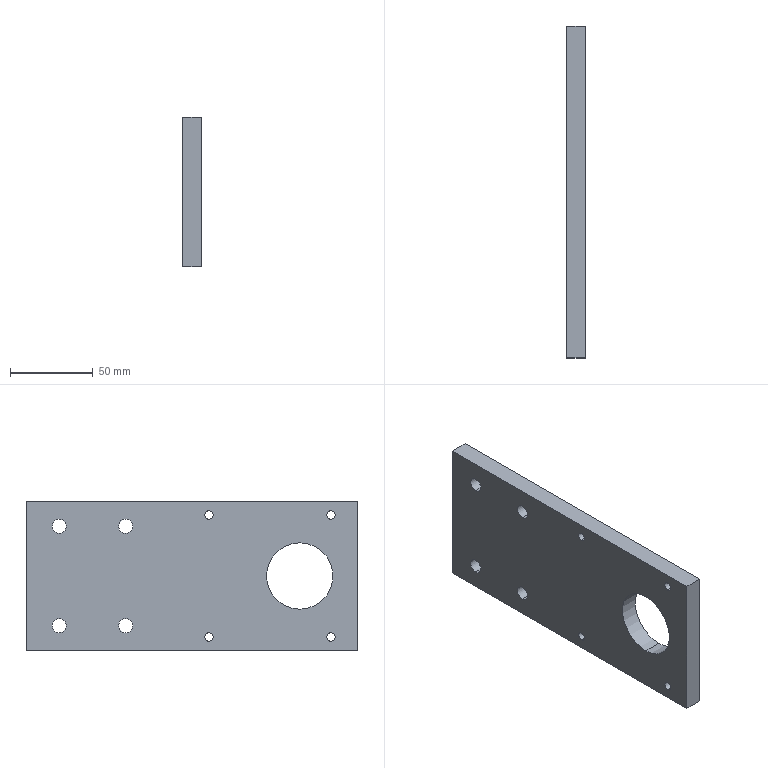Part | STEP file | PN_0021 (drive mounting plate) | 1 solid | 24 faces | box 11 x 200 x 90 mm | volume 180816 mm3 | cylinder 18 | plane 6 | commonest cylinder face diameters 5 x8 8.5 x8 40 x2